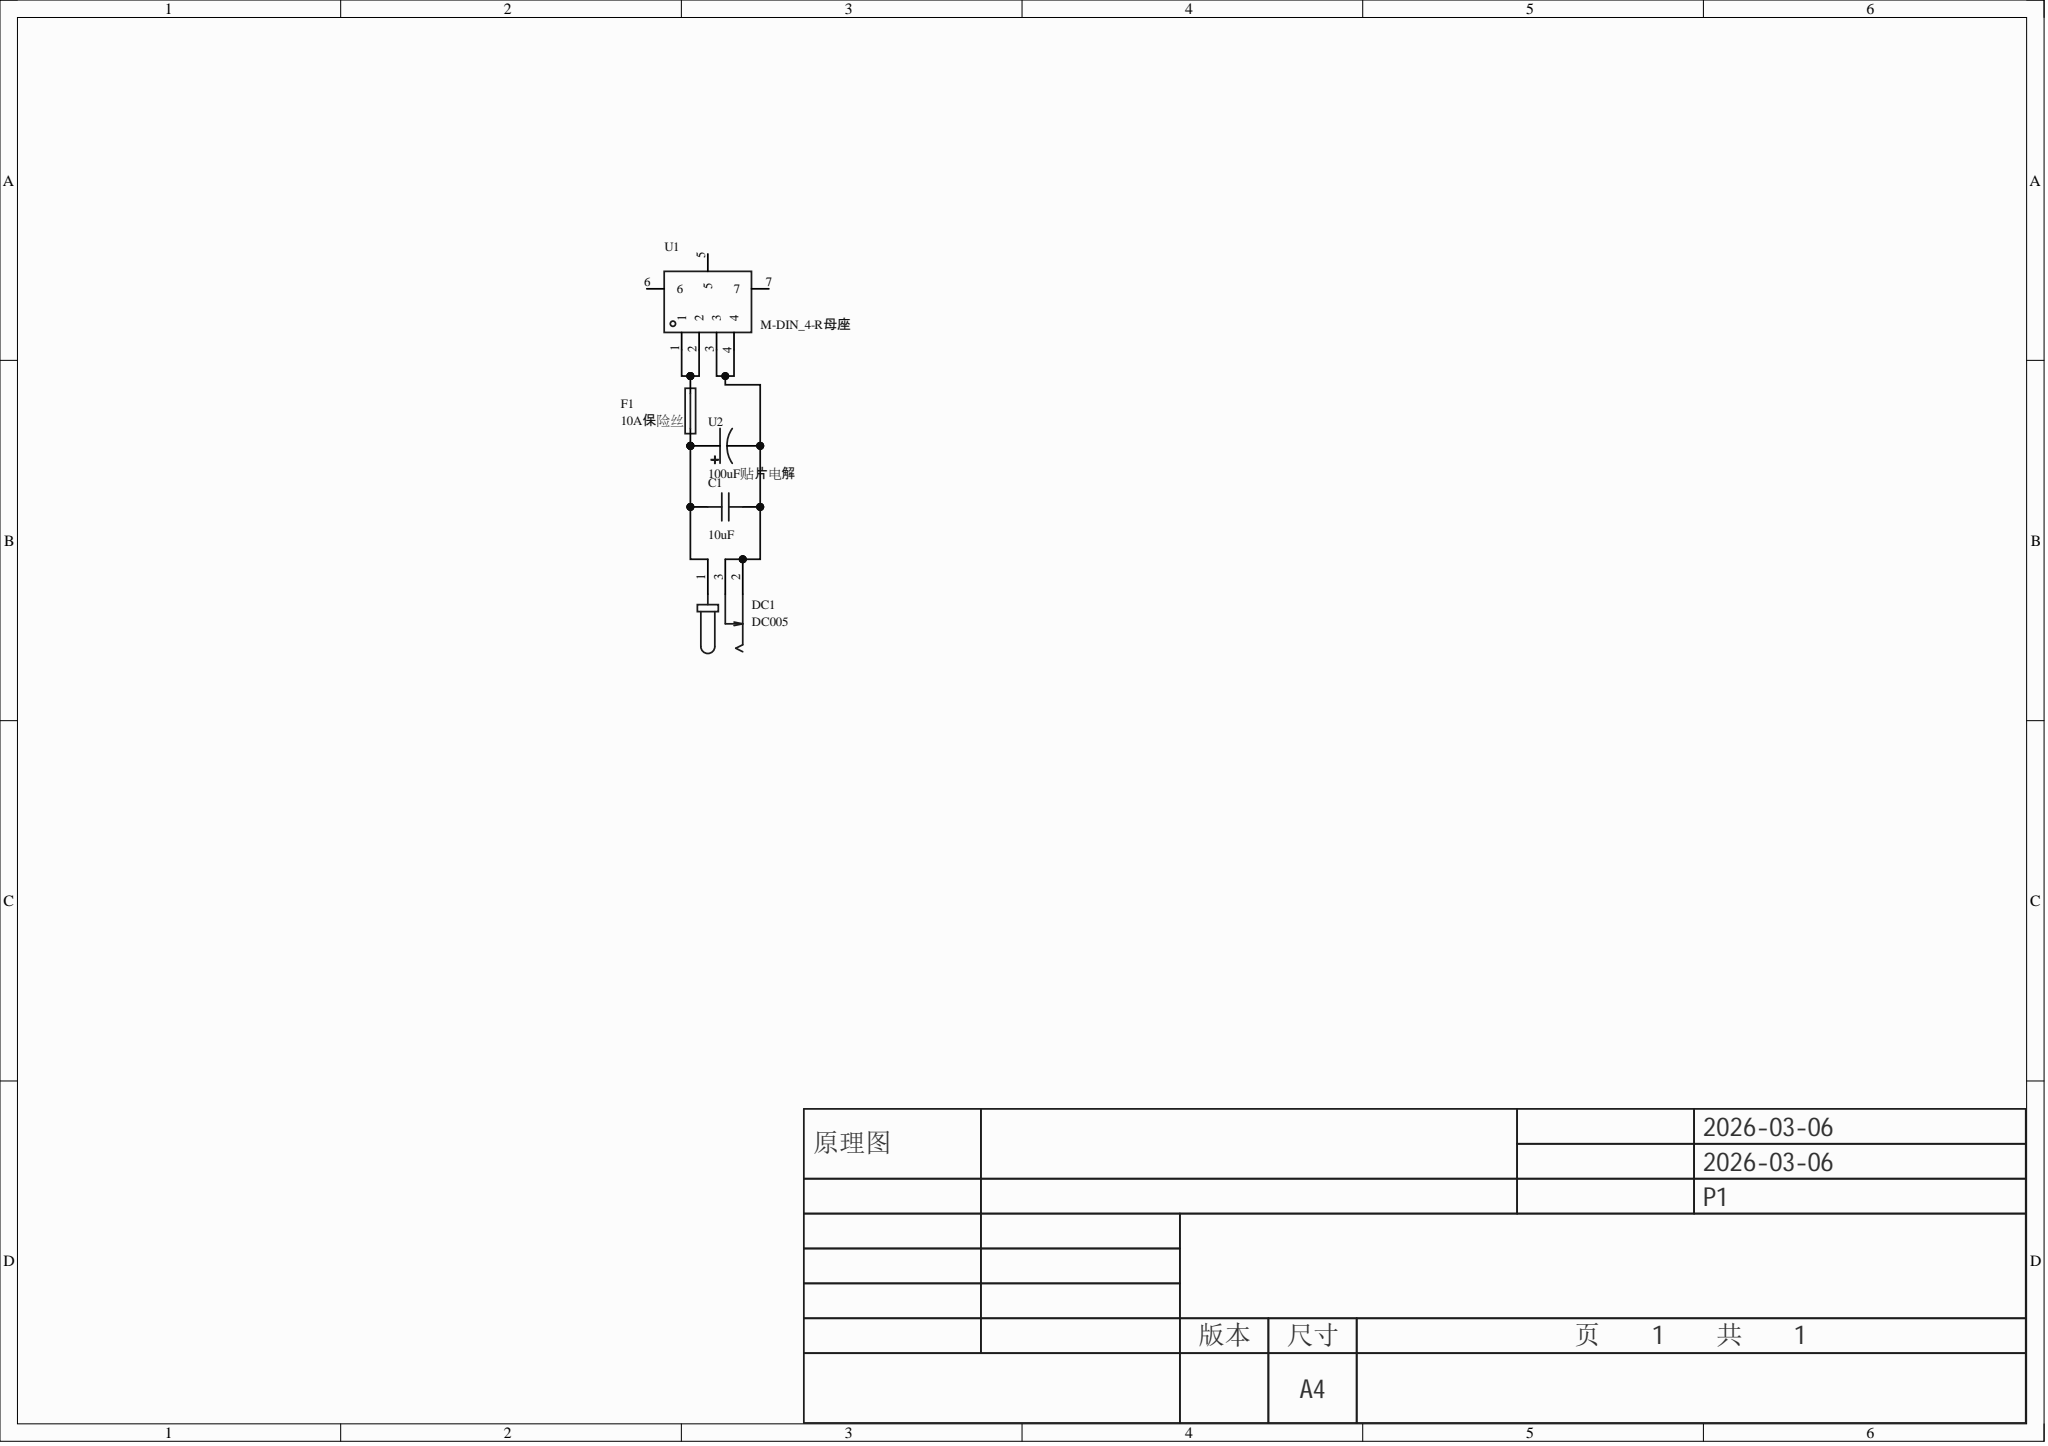Circuit board | Altium Designer | 5 parts | 3 nets
Bill of materials:
Comment,Description,Designator,Footprint,LibRef,Quantity
"10uF","","C1","C0603","CAP_0603","1"
"DC005","连接器类型:DC电源插座;安装方式:弯插;触点内径:2mm;触点外径:6.3mm;额定电流:500mA;额定电压:12V;工作温度:-30℃~+70℃;","DC1","DC-IN-TH_DC005","DC005","1"
"10A保险丝","","F1","FUSE-SMD_L6.1-W2.6","10A保险丝","1"
"M-DIN_4-R母座","","U1","CONN-TH_DIN_4P_12D8","M-DIN_4-R母座","1"
"100uF贴片电解","","U2","CAP-SMD_BD6.3-L6.6-W6.6-LS7.4-FD","100uF贴片电解","1"
Netlist (Protel format):
[
C1
C0603
10uF



]
[
DC1
DC-IN-TH_DC005
DC005



]
[
F1
FUSE-SMD_L6.1-W2.6
10A保险丝



]
[
U1
CONN-TH_DIN_4P_12D8
M-DIN_4-R母座



]
[
U2
CAP-SMD_BD6.3-L6.6-W6.6-LS7.4-FD
100uF贴片电解



]
(
NetF1_2
F1-2
U1-1
U1-2
)
(
NetC1_2
C1-2
DC1-2
DC1-3
U1-3
U1-4
U2-2
)
(
NetC1_1
C1-1
DC1-1
F1-1
U2-1
)